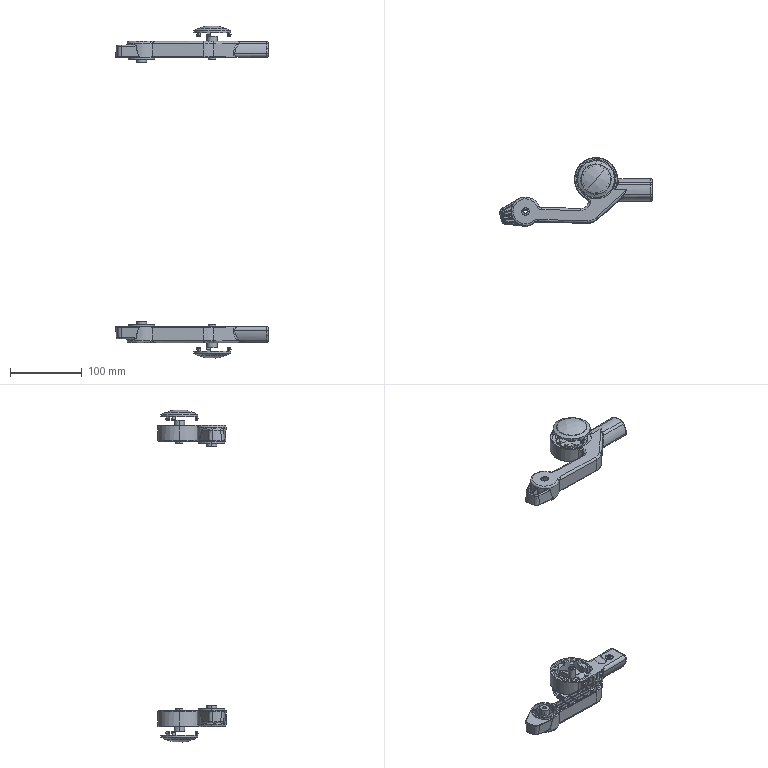Part | SolidWorks | 6 solids | 1561 faces | box 212.741 x 95 x 464 mm | volume 193426 mm3 | plane 644 | cylinder 434 | spline 369 | torus 60 | sphere 42 | cone 12 | commonest cylinder face diameters 1 x66 37 x30 54 x20 2 x19 4 x18 46 x14